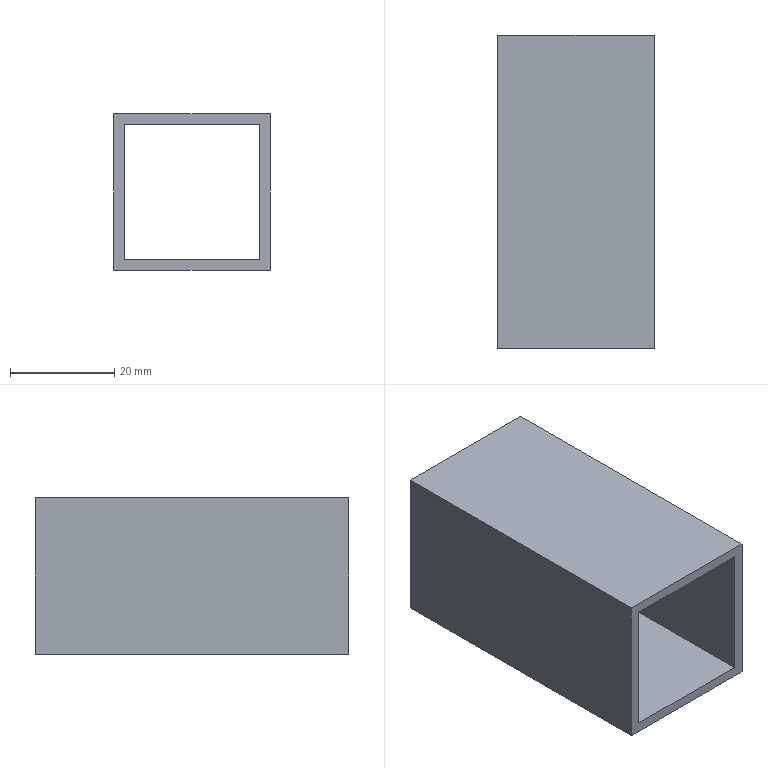Part | NX | features solid 2 | 1 solid | 10 faces | box 30 x 60 x 30 mm | volume 13440 mm3 | plane 10
STEP:
#1=CARTESIAN_POINT('',(635.,-528.785,-135.));
#2=VERTEX_POINT('',#1);
#3=CARTESIAN_POINT('',(635.,-528.785,-105.));
#4=VERTEX_POINT('',#3);
#5=CARTESIAN_POINT('',(635.,-528.785,-135.));
#6=DIRECTION('',(0.,0.,1.));
#7=VECTOR('',#6,1000.);
#8=LINE('',#5,#7);
#9=EDGE_CURVE('',#2,#4,#8,.T.);
#10=ORIENTED_EDGE('',*,*,#9,.F.);
#11=CARTESIAN_POINT('',(635.,-588.785,-135.));
#12=VERTEX_POINT('',#11);
#13=CARTESIAN_POINT('',(635.,-568.785,-135.));
#14=DIRECTION('',(0.,-1.,0.));
#15=VECTOR('',#14,1000.);
#16=LINE('',#13,#15);
#17=EDGE_CURVE('',#12,#2,#16,.F.);
#18=ORIENTED_EDGE('',*,*,#17,.F.);
#19=CARTESIAN_POINT('',(635.,-588.785,-105.));
#20=VERTEX_POINT('',#19);
#21=CARTESIAN_POINT('',(635.,-588.785,-135.));
#22=DIRECTION('',(0.,0.,-1.));
#23=VECTOR('',#22,1000.);
#24=LINE('',#21,#23);
#25=EDGE_CURVE('',#20,#12,#24,.T.);
#26=ORIENTED_EDGE('',*,*,#25,.F.);
#27=CARTESIAN_POINT('',(635.,-568.785,-105.));
#28=DIRECTION('',(0.,-1.,0.));
#29=VECTOR('',#28,1000.);
#30=LINE('',#27,#29);
#31=EDGE_CURVE('',#20,#4,#30,.F.);
#32=ORIENTED_EDGE('',*,*,#31,.T.);
#33=EDGE_LOOP('',(#10,#18,#26,#32));
#34=FACE_BOUND('',#33,.T.);
#35=CARTESIAN_POINT('',(635.,-568.785,-135.));
#36=DIRECTION('',(1.,0.,0.));
#37=DIRECTION('',(0.,0.,-1.));
#38=AXIS2_PLACEMENT_3D('',#35,#36,#37);
#39=PLANE('',#38);
#40=ADVANCED_FACE('',(#34),#39,.F.);
#41=CARTESIAN_POINT('',(665.,-588.785,-135.));
#42=VERTEX_POINT('',#41);
#43=CARTESIAN_POINT('',(665.,-528.785,-135.));
#44=VERTEX_POINT('',#43);
#45=CARTESIAN_POINT('',(665.,-568.785,-135.));
#46=DIRECTION('',(0.,1.,0.));
#47=VECTOR('',#46,1000.);
#48=LINE('',#45,#47);
#49=EDGE_CURVE('',#42,#44,#48,.T.);
#50=ORIENTED_EDGE('',*,*,#49,.T.);
#51=CARTESIAN_POINT('',(665.,-528.785,-105.));
#52=VERTEX_POINT('',#51);
#53=CARTESIAN_POINT('',(665.,-528.785,-135.));
#54=DIRECTION('',(0.,0.,1.));
#55=VECTOR('',#54,1000.);
#56=LINE('',#53,#55);
#57=EDGE_CURVE('',#44,#52,#56,.T.);
#58=ORIENTED_EDGE('',*,*,#57,.T.);
#59=CARTESIAN_POINT('',(665.,-588.785,-105.));
#60=VERTEX_POINT('',#59);
#61=CARTESIAN_POINT('',(665.,-568.785,-105.));
#62=DIRECTION('',(0.,1.,0.));
#63=VECTOR('',#62,1000.);
#64=LINE('',#61,#63);
#65=EDGE_CURVE('',#60,#52,#64,.T.);
#66=ORIENTED_EDGE('',*,*,#65,.F.);
#67=CARTESIAN_POINT('',(665.,-588.785,-135.));
#68=DIRECTION('',(0.,0.,-1.));
#69=VECTOR('',#68,1000.);
#70=LINE('',#67,#69);
#71=EDGE_CURVE('',#60,#42,#70,.T.);
#72=ORIENTED_EDGE('',*,*,#71,.T.);
#73=EDGE_LOOP('',(#50,#58,#66,#72));
#74=FACE_BOUND('',#73,.T.);
#75=CARTESIAN_POINT('',(665.,-568.785,-135.));
#76=DIRECTION('',(1.,0.,0.));
#77=DIRECTION('',(0.,0.,-1.));
#78=AXIS2_PLACEMENT_3D('',#75,#76,#77);
#79=PLANE('',#78);
#80=ADVANCED_FACE('',(#74),#79,.T.);
#81=CARTESIAN_POINT('',(675.,-528.785,-105.));
#82=DIRECTION('',(1.,0.,0.));
#83=VECTOR('',#82,1000.);
#84=LINE('',#81,#83);
#85=EDGE_CURVE('',#4,#52,#84,.T.);
#86=ORIENTED_EDGE('',*,*,#85,.F.);
#87=ORIENTED_EDGE('',*,*,#31,.F.);
#88=CARTESIAN_POINT('',(675.,-588.785,-105.));
#89=DIRECTION('',(-1.,0.,0.));
#90=VECTOR('',#89,1000.);
#91=LINE('',#88,#90);
#92=EDGE_CURVE('',#60,#20,#91,.T.);
#93=ORIENTED_EDGE('',*,*,#92,.F.);
#94=ORIENTED_EDGE('',*,*,#65,.T.);
#95=EDGE_LOOP('',(#86,#87,#93,#94));
#96=FACE_BOUND('',#95,.T.);
#97=CARTESIAN_POINT('',(675.,-568.785,-105.));
#98=DIRECTION('',(0.,0.,-1.));
#99=DIRECTION('',(-1.,0.,0.));
#100=AXIS2_PLACEMENT_3D('',#97,#98,#99);
#101=PLANE('',#100);
#102=ADVANCED_FACE('',(#96),#101,.F.);
#103=ORIENTED_EDGE('',*,*,#17,.T.);
#104=CARTESIAN_POINT('',(675.,-528.785,-135.));
#105=DIRECTION('',(1.,0.,0.));
#106=VECTOR('',#105,1000.);
#107=LINE('',#104,#106);
#108=EDGE_CURVE('',#2,#44,#107,.T.);
#109=ORIENTED_EDGE('',*,*,#108,.T.);
#110=ORIENTED_EDGE('',*,*,#49,.F.);
#111=CARTESIAN_POINT('',(675.,-588.785,-135.));
#112=DIRECTION('',(-1.,0.,0.));
#113=VECTOR('',#112,1000.);
#114=LINE('',#111,#113);
#115=EDGE_CURVE('',#42,#12,#114,.T.);
#116=ORIENTED_EDGE('',*,*,#115,.T.);
#117=EDGE_LOOP('',(#103,#109,#110,#116));
#118=FACE_BOUND('',#117,.T.);
#119=CARTESIAN_POINT('',(675.,-568.785,-135.));
#120=DIRECTION('',(0.,0.,-1.));
#121=DIRECTION('',(-1.,0.,0.));
#122=AXIS2_PLACEMENT_3D('',#119,#120,#121);
#123=PLANE('',#122);
#124=ADVANCED_FACE('',(#118),#123,.T.);
#125=CARTESIAN_POINT('',(637.,-588.785,-133.));
#126=VERTEX_POINT('',#125);
#127=CARTESIAN_POINT('',(637.,-528.785,-133.));
#128=VERTEX_POINT('',#127);
#129=CARTESIAN_POINT('',(637.,-568.785,-133.));
#130=DIRECTION('',(0.,1.,0.));
#131=VECTOR('',#130,1000.);
#132=LINE('',#129,#131);
#133=EDGE_CURVE('',#126,#128,#132,.T.);
#134=ORIENTED_EDGE('',*,*,#133,.T.);
#135=CARTESIAN_POINT('',(637.,-528.785,-107.));
#136=VERTEX_POINT('',#135);
#137=CARTESIAN_POINT('',(637.,-528.785,-135.));
#138=DIRECTION('',(0.,0.,1.));
#139=VECTOR('',#138,1000.);
#140=LINE('',#137,#139);
#141=EDGE_CURVE('',#128,#136,#140,.T.);
#142=ORIENTED_EDGE('',*,*,#141,.T.);
#143=CARTESIAN_POINT('',(637.,-588.785,-107.));
#144=VERTEX_POINT('',#143);
#145=CARTESIAN_POINT('',(637.,-568.785,-107.));
#146=DIRECTION('',(0.,1.,0.));
#147=VECTOR('',#146,1000.);
#148=LINE('',#145,#147);
#149=EDGE_CURVE('',#144,#136,#148,.T.);
#150=ORIENTED_EDGE('',*,*,#149,.F.);
#151=CARTESIAN_POINT('',(637.,-588.785,-135.));
#152=DIRECTION('',(0.,0.,-1.));
#153=VECTOR('',#152,1000.);
#154=LINE('',#151,#153);
#155=EDGE_CURVE('',#144,#126,#154,.T.);
#156=ORIENTED_EDGE('',*,*,#155,.T.);
#157=EDGE_LOOP('',(#134,#142,#150,#156));
#158=FACE_BOUND('',#157,.T.);
#159=CARTESIAN_POINT('',(637.,-568.785,-135.));
#160=DIRECTION('',(1.,0.,0.));
#161=DIRECTION('',(0.,0.,-1.));
#162=AXIS2_PLACEMENT_3D('',#159,#160,#161);
#163=PLANE('',#162);
#164=ADVANCED_FACE('',(#158),#163,.T.);
#165=CARTESIAN_POINT('',(663.,-528.785,-133.));
#166=VERTEX_POINT('',#165);
#167=CARTESIAN_POINT('',(663.,-528.785,-107.));
#168=VERTEX_POINT('',#167);
#169=CARTESIAN_POINT('',(663.,-528.785,-135.));
#170=DIRECTION('',(0.,0.,1.));
#171=VECTOR('',#170,1000.);
#172=LINE('',#169,#171);
#173=EDGE_CURVE('',#166,#168,#172,.T.);
#174=ORIENTED_EDGE('',*,*,#173,.F.);
#175=CARTESIAN_POINT('',(663.,-588.785,-133.));
#176=VERTEX_POINT('',#175);
#177=CARTESIAN_POINT('',(663.,-568.785,-133.));
#178=DIRECTION('',(0.,1.,0.));
#179=VECTOR('',#178,1000.);
#180=LINE('',#177,#179);
#181=EDGE_CURVE('',#176,#166,#180,.T.);
#182=ORIENTED_EDGE('',*,*,#181,.F.);
#183=CARTESIAN_POINT('',(663.,-588.785,-107.));
#184=VERTEX_POINT('',#183);
#185=CARTESIAN_POINT('',(663.,-588.785,-135.));
#186=DIRECTION('',(0.,0.,-1.));
#187=VECTOR('',#186,1000.);
#188=LINE('',#185,#187);
#189=EDGE_CURVE('',#184,#176,#188,.T.);
#190=ORIENTED_EDGE('',*,*,#189,.F.);
#191=CARTESIAN_POINT('',(663.,-568.785,-107.));
#192=DIRECTION('',(0.,1.,0.));
#193=VECTOR('',#192,1000.);
#194=LINE('',#191,#193);
#195=EDGE_CURVE('',#184,#168,#194,.T.);
#196=ORIENTED_EDGE('',*,*,#195,.T.);
#197=EDGE_LOOP('',(#174,#182,#190,#196));
#198=FACE_BOUND('',#197,.T.);
#199=CARTESIAN_POINT('',(663.,-568.785,-135.));
#200=DIRECTION('',(1.,0.,0.));
#201=DIRECTION('',(0.,0.,-1.));
#202=AXIS2_PLACEMENT_3D('',#199,#200,#201);
#203=PLANE('',#202);
#204=ADVANCED_FACE('',(#198),#203,.F.);
#205=ORIENTED_EDGE('',*,*,#149,.T.);
#206=CARTESIAN_POINT('',(675.,-528.785,-107.));
#207=DIRECTION('',(1.,0.,0.));
#208=VECTOR('',#207,1000.);
#209=LINE('',#206,#208);
#210=EDGE_CURVE('',#136,#168,#209,.T.);
#211=ORIENTED_EDGE('',*,*,#210,.T.);
#212=ORIENTED_EDGE('',*,*,#195,.F.);
#213=CARTESIAN_POINT('',(675.,-588.785,-107.));
#214=DIRECTION('',(-1.,0.,0.));
#215=VECTOR('',#214,1000.);
#216=LINE('',#213,#215);
#217=EDGE_CURVE('',#184,#144,#216,.T.);
#218=ORIENTED_EDGE('',*,*,#217,.T.);
#219=EDGE_LOOP('',(#205,#211,#212,#218));
#220=FACE_BOUND('',#219,.T.);
#221=CARTESIAN_POINT('',(675.,-568.785,-107.));
#222=DIRECTION('',(0.,0.,-1.));
#223=DIRECTION('',(-1.,0.,0.));
#224=AXIS2_PLACEMENT_3D('',#221,#222,#223);
#225=PLANE('',#224);
#226=ADVANCED_FACE('',(#220),#225,.T.);
#227=CARTESIAN_POINT('',(675.,-528.785,-133.));
#228=DIRECTION('',(1.,0.,0.));
#229=VECTOR('',#228,1000.);
#230=LINE('',#227,#229);
#231=EDGE_CURVE('',#128,#166,#230,.T.);
#232=ORIENTED_EDGE('',*,*,#231,.F.);
#233=ORIENTED_EDGE('',*,*,#133,.F.);
#234=CARTESIAN_POINT('',(675.,-588.785,-133.));
#235=DIRECTION('',(-1.,0.,0.));
#236=VECTOR('',#235,1000.);
#237=LINE('',#234,#236);
#238=EDGE_CURVE('',#176,#126,#237,.T.);
#239=ORIENTED_EDGE('',*,*,#238,.F.);
#240=ORIENTED_EDGE('',*,*,#181,.T.);
#241=EDGE_LOOP('',(#232,#233,#239,#240));
#242=FACE_BOUND('',#241,.T.);
#243=CARTESIAN_POINT('',(675.,-568.785,-133.));
#244=DIRECTION('',(0.,0.,-1.));
#245=DIRECTION('',(-1.,0.,0.));
#246=AXIS2_PLACEMENT_3D('',#243,#244,#245);
#247=PLANE('',#246);
#248=ADVANCED_FACE('',(#242),#247,.F.);
#249=ORIENTED_EDGE('',*,*,#115,.F.);
#250=ORIENTED_EDGE('',*,*,#71,.F.);
#251=ORIENTED_EDGE('',*,*,#92,.T.);
#252=ORIENTED_EDGE('',*,*,#25,.T.);
#253=EDGE_LOOP('',(#249,#250,#251,#252));
#254=FACE_BOUND('',#253,.T.);
#255=ORIENTED_EDGE('',*,*,#189,.T.);
#256=ORIENTED_EDGE('',*,*,#238,.T.);
#257=ORIENTED_EDGE('',*,*,#155,.F.);
#258=ORIENTED_EDGE('',*,*,#217,.F.);
#259=EDGE_LOOP('',(#255,#256,#257,#258));
#260=FACE_BOUND('',#259,.T.);
#261=CARTESIAN_POINT('',(675.,-588.785,-105.));
#262=DIRECTION('',(0.,-1.,0.));
#263=DIRECTION('',(-1.,0.,0.));
#264=AXIS2_PLACEMENT_3D('',#261,#262,#263);
#265=PLANE('',#264);
#266=ADVANCED_FACE('',(#254,#260),#265,.T.);
#267=ORIENTED_EDGE('',*,*,#210,.F.);
#268=ORIENTED_EDGE('',*,*,#141,.F.);
#269=ORIENTED_EDGE('',*,*,#231,.T.);
#270=ORIENTED_EDGE('',*,*,#173,.T.);
#271=EDGE_LOOP('',(#267,#268,#269,#270));
#272=FACE_BOUND('',#271,.T.);
#273=ORIENTED_EDGE('',*,*,#9,.T.);
#274=ORIENTED_EDGE('',*,*,#85,.T.);
#275=ORIENTED_EDGE('',*,*,#57,.F.);
#276=ORIENTED_EDGE('',*,*,#108,.F.);
#277=EDGE_LOOP('',(#273,#274,#275,#276));
#278=FACE_BOUND('',#277,.T.);
#279=CARTESIAN_POINT('',(635.,-528.785,-105.));
#280=DIRECTION('',(0.,1.,0.));
#281=DIRECTION('',(0.,0.,1.));
#282=AXIS2_PLACEMENT_3D('',#279,#280,#281);
#283=PLANE('',#282);
#284=ADVANCED_FACE('',(#272,#278),#283,.T.);
#285=CLOSED_SHELL('',(#40,#80,#102,#124,#164,#204,#226,#248,#266,#284));
#286=MANIFOLD_SOLID_BREP('',#285);
#287=(LENGTH_UNIT()NAMED_UNIT(*)SI_UNIT(.MILLI.,.METRE.));
#288=UNCERTAINTY_MEASURE_WITH_UNIT(LENGTH_MEASURE(0.00001),#287,'','');
#289=(NAMED_UNIT(*)PLANE_ANGLE_UNIT()SI_UNIT($,.RADIAN.));
#290=(NAMED_UNIT(*)SI_UNIT($,.STERADIAN.)SOLID_ANGLE_UNIT());
#291=(GEOMETRIC_REPRESENTATION_CONTEXT(3)GLOBAL_UNCERTAINTY_ASSIGNED_CONTEXT((#288))GLOBAL_UNIT_ASSIGNED_CONTEXT((#287,#289,#290))REPRESENTATION_CONTEXT('',''));
#292=ADVANCED_BREP_SHAPE_REPRESENTATION('',(#286),#291);